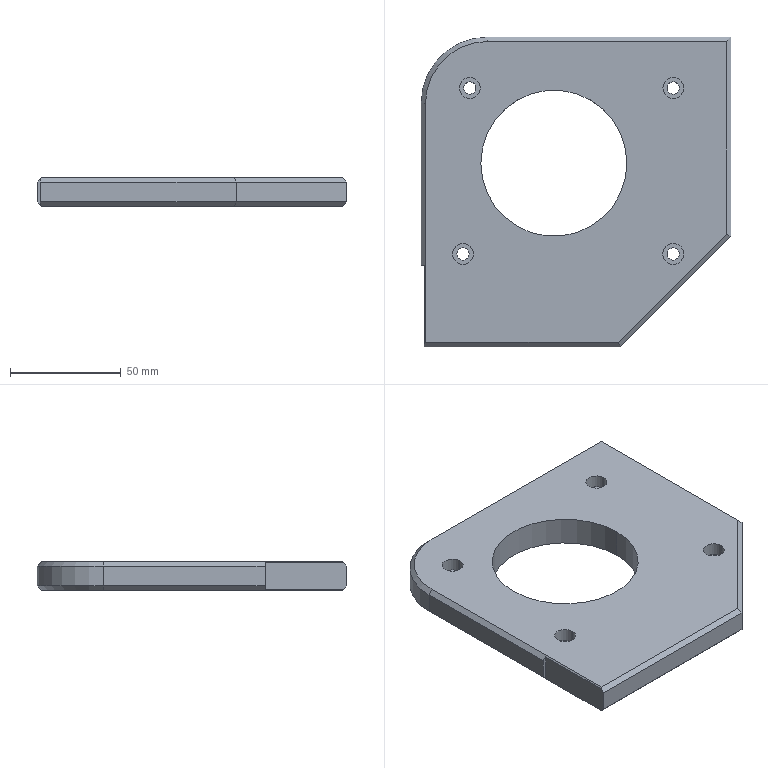Part | Creo | 1 solid | 44 faces | box 140 x 140 x 13 mm | volume 186564 mm3 | plane 23 | cylinder 19 | cone 2 | commonest cylinder face diameters 5.5 x8 9.5 x8 66 x2 60 x1
STEP:
#1=CARTESIAN_POINT('',(196.5,-375.005,-22.));
#2=VERTEX_POINT('',#1);
#3=CARTESIAN_POINT('',(196.5,-375.005,-13.));
#4=VERTEX_POINT('',#3);
#5=CARTESIAN_POINT('',(196.5,-375.005,-22.));
#6=DIRECTION('',(0.,0.,1.));
#7=VECTOR('',#6,9.);
#8=LINE('',#5,#7);
#9=EDGE_CURVE('',#2,#4,#8,.T.);
#10=ORIENTED_EDGE('',*,*,#9,.T.);
#11=CARTESIAN_POINT('',(285.,-375.005,-13.));
#12=VERTEX_POINT('',#11);
#13=CARTESIAN_POINT('',(196.5,-375.005,-13.));
#14=DIRECTION('',(1.,0.,0.));
#15=VECTOR('',#14,88.5);
#16=LINE('',#13,#15);
#17=EDGE_CURVE('',#4,#12,#16,.T.);
#18=ORIENTED_EDGE('',*,*,#17,.T.);
#19=CARTESIAN_POINT('',(285.,-375.005,-22.));
#20=VERTEX_POINT('',#19);
#21=CARTESIAN_POINT('',(285.,-375.005,-13.));
#22=DIRECTION('',(0.,0.,-1.));
#23=VECTOR('',#22,9.);
#24=LINE('',#21,#23);
#25=EDGE_CURVE('',#12,#20,#24,.T.);
#26=ORIENTED_EDGE('',*,*,#25,.T.);
#27=CARTESIAN_POINT('',(285.,-375.005,-22.));
#28=DIRECTION('',(-1.,0.,0.));
#29=VECTOR('',#28,88.5);
#30=LINE('',#27,#29);
#31=EDGE_CURVE('',#20,#2,#30,.T.);
#32=ORIENTED_EDGE('',*,*,#31,.T.);
#33=EDGE_LOOP('',(#10,#18,#26,#32));
#34=FACE_OUTER_BOUND('',#33,.F.);
#35=CARTESIAN_POINT('',(-265.,-375.005,-187.));
#36=DIRECTION('',(0.,-1.,0.));
#37=DIRECTION('',(0.,0.,1.));
#38=AXIS2_PLACEMENT_3D('',#35,#36,#37);
#39=PLANE('',#38);
#40=ADVANCED_FACE('',(#34),#39,.T.);
#41=CARTESIAN_POINT('',(196.5,-338.005,-11.5));
#42=VERTEX_POINT('',#41);
#43=CARTESIAN_POINT('',(196.5,-338.005,-23.5));
#44=VERTEX_POINT('',#43);
#45=CARTESIAN_POINT('',(196.5,-338.005,-11.5));
#46=DIRECTION('',(0.,0.,-1.));
#47=VECTOR('',#46,12.);
#48=LINE('',#45,#47);
#49=EDGE_CURVE('',#42,#44,#48,.T.);
#50=ORIENTED_EDGE('',*,*,#49,.F.);
#51=CARTESIAN_POINT('',(196.5,-373.505,-11.5));
#52=VERTEX_POINT('',#51);
#53=CARTESIAN_POINT('',(196.5,-338.005,-11.5));
#54=DIRECTION('',(0.,-1.,0.));
#55=VECTOR('',#54,35.5);
#56=LINE('',#53,#55);
#57=EDGE_CURVE('',#42,#52,#56,.T.);
#58=ORIENTED_EDGE('',*,*,#57,.T.);
#59=CARTESIAN_POINT('',(196.5,-375.005,-13.));
#60=DIRECTION('',(0.,0.7071,0.7071));
#61=VECTOR('',#60,2.121);
#62=LINE('',#59,#61);
#63=EDGE_CURVE('',#4,#52,#62,.T.);
#64=ORIENTED_EDGE('',*,*,#63,.F.);
#65=ORIENTED_EDGE('',*,*,#9,.F.);
#66=CARTESIAN_POINT('',(196.5,-373.505,-23.5));
#67=VERTEX_POINT('',#66);
#68=CARTESIAN_POINT('',(196.5,-373.505,-23.5));
#69=DIRECTION('',(0.,-0.7071,0.7071));
#70=VECTOR('',#69,2.121);
#71=LINE('',#68,#70);
#72=EDGE_CURVE('',#67,#2,#71,.T.);
#73=ORIENTED_EDGE('',*,*,#72,.F.);
#74=CARTESIAN_POINT('',(196.5,-373.505,-23.5));
#75=DIRECTION('',(0.,1.,0.));
#76=VECTOR('',#75,35.5);
#77=LINE('',#74,#76);
#78=EDGE_CURVE('',#67,#44,#77,.T.);
#79=ORIENTED_EDGE('',*,*,#78,.T.);
#80=EDGE_LOOP('',(#50,#58,#64,#65,#73,#79));
#81=FACE_OUTER_BOUND('',#80,.F.);
#82=CARTESIAN_POINT('',(196.5,-394.005,172.076));
#83=DIRECTION('',(1.,0.,0.));
#84=DIRECTION('',(0.,0.,-1.));
#85=AXIS2_PLACEMENT_3D('',#82,#83,#84);
#86=PLANE('',#85);
#87=ADVANCED_FACE('',(#81),#86,.F.);
#88=CARTESIAN_POINT('',(195.,-338.005,-13.));
#89=VERTEX_POINT('',#88);
#90=CARTESIAN_POINT('',(195.,-338.005,-22.));
#91=VERTEX_POINT('',#90);
#92=CARTESIAN_POINT('',(195.,-338.005,-13.));
#93=DIRECTION('',(0.,0.,-1.));
#94=VECTOR('',#93,9.);
#95=LINE('',#92,#94);
#96=EDGE_CURVE('',#89,#91,#95,.T.);
#97=ORIENTED_EDGE('',*,*,#96,.F.);
#98=CARTESIAN_POINT('',(196.5,-338.005,-11.5));
#99=DIRECTION('',(-0.7071,0.,-0.7071));
#100=VECTOR('',#99,2.121);
#101=LINE('',#98,#100);
#102=EDGE_CURVE('',#42,#89,#101,.T.);
#103=ORIENTED_EDGE('',*,*,#102,.F.);
#104=ORIENTED_EDGE('',*,*,#49,.T.);
#105=CARTESIAN_POINT('',(195.,-338.005,-22.));
#106=DIRECTION('',(0.7071,0.,-0.7071));
#107=VECTOR('',#106,2.121);
#108=LINE('',#105,#107);
#109=EDGE_CURVE('',#91,#44,#108,.T.);
#110=ORIENTED_EDGE('',*,*,#109,.F.);
#111=EDGE_LOOP('',(#97,#103,#104,#110));
#112=FACE_OUTER_BOUND('',#111,.F.);
#113=CARTESIAN_POINT('',(175.,-338.005,-2.));
#114=DIRECTION('',(0.,-1.,0.));
#115=DIRECTION('',(1.,0.,0.));
#116=AXIS2_PLACEMENT_3D('',#113,#114,#115);
#117=PLANE('',#116);
#118=ADVANCED_FACE('',(#112),#117,.T.);
#119=CARTESIAN_POINT('',(195.,-265.005,-22.));
#120=VERTEX_POINT('',#119);
#121=CARTESIAN_POINT('',(195.,-265.005,-13.));
#122=VERTEX_POINT('',#121);
#123=CARTESIAN_POINT('',(195.,-265.005,-22.));
#124=DIRECTION('',(0.,0.,1.));
#125=VECTOR('',#124,9.);
#126=LINE('',#123,#125);
#127=EDGE_CURVE('',#120,#122,#126,.T.);
#128=ORIENTED_EDGE('',*,*,#127,.T.);
#129=CARTESIAN_POINT('',(195.,-265.005,-13.));
#130=DIRECTION('',(0.,-1.,0.));
#131=VECTOR('',#130,73.);
#132=LINE('',#129,#131);
#133=EDGE_CURVE('',#122,#89,#132,.T.);
#134=ORIENTED_EDGE('',*,*,#133,.T.);
#135=ORIENTED_EDGE('',*,*,#96,.T.);
#136=CARTESIAN_POINT('',(195.,-338.005,-22.));
#137=DIRECTION('',(0.,1.,0.));
#138=VECTOR('',#137,73.);
#139=LINE('',#136,#138);
#140=EDGE_CURVE('',#91,#120,#139,.T.);
#141=ORIENTED_EDGE('',*,*,#140,.T.);
#142=EDGE_LOOP('',(#128,#134,#135,#141));
#143=FACE_OUTER_BOUND('',#142,.F.);
#144=CARTESIAN_POINT('',(195.,-0.004699,-23.));
#145=DIRECTION('',(1.,0.,0.));
#146=DIRECTION('',(0.,-1.,0.));
#147=AXIS2_PLACEMENT_3D('',#144,#145,#146);
#148=PLANE('',#147);
#149=ADVANCED_FACE('',(#143),#148,.F.);
#150=CARTESIAN_POINT('',(225.,-235.005,-13.));
#151=VERTEX_POINT('',#150);
#152=CARTESIAN_POINT('',(225.,-235.005,-22.));
#153=VERTEX_POINT('',#152);
#154=CARTESIAN_POINT('',(225.,-235.005,-13.));
#155=DIRECTION('',(0.,0.,-1.));
#156=VECTOR('',#155,9.);
#157=LINE('',#154,#156);
#158=EDGE_CURVE('',#151,#153,#157,.T.);
#159=ORIENTED_EDGE('',*,*,#158,.F.);
#160=CARTESIAN_POINT('',(225.,-265.005,-13.));
#161=DIRECTION('',(0.,0.,1.));
#162=DIRECTION('',(0.,1.,0.));
#163=AXIS2_PLACEMENT_3D('',#160,#161,#162);
#164=CIRCLE('',#163,30.);
#165=EDGE_CURVE('',#151,#122,#164,.T.);
#166=ORIENTED_EDGE('',*,*,#165,.T.);
#167=ORIENTED_EDGE('',*,*,#127,.F.);
#168=CARTESIAN_POINT('',(225.,-265.005,-22.));
#169=DIRECTION('',(0.,0.,-1.));
#170=DIRECTION('',(-1.,0.,0.));
#171=AXIS2_PLACEMENT_3D('',#168,#169,#170);
#172=CIRCLE('',#171,30.);
#173=EDGE_CURVE('',#120,#153,#172,.T.);
#174=ORIENTED_EDGE('',*,*,#173,.T.);
#175=EDGE_LOOP('',(#159,#166,#167,#174));
#176=FACE_OUTER_BOUND('',#175,.F.);
#177=CARTESIAN_POINT('',(225.,-265.005,-12.));
#178=DIRECTION('',(0.,0.,1.));
#179=DIRECTION('',(-1.,0.,0.));
#180=AXIS2_PLACEMENT_3D('',#177,#178,#179);
#181=CYLINDRICAL_SURFACE('',#180,30.);
#182=ADVANCED_FACE('',(#176),#181,.T.);
#183=CARTESIAN_POINT('',(335.,-235.005,-22.));
#184=VERTEX_POINT('',#183);
#185=CARTESIAN_POINT('',(335.,-235.005,-13.));
#186=VERTEX_POINT('',#185);
#187=CARTESIAN_POINT('',(335.,-235.005,-22.));
#188=DIRECTION('',(0.,0.,1.));
#189=VECTOR('',#188,9.);
#190=LINE('',#187,#189);
#191=EDGE_CURVE('',#184,#186,#190,.T.);
#192=ORIENTED_EDGE('',*,*,#191,.T.);
#193=CARTESIAN_POINT('',(335.,-235.005,-13.));
#194=DIRECTION('',(-1.,0.,0.));
#195=VECTOR('',#194,110.);
#196=LINE('',#193,#195);
#197=EDGE_CURVE('',#186,#151,#196,.T.);
#198=ORIENTED_EDGE('',*,*,#197,.T.);
#199=ORIENTED_EDGE('',*,*,#158,.T.);
#200=CARTESIAN_POINT('',(225.,-235.005,-22.));
#201=DIRECTION('',(1.,0.,0.));
#202=VECTOR('',#201,110.);
#203=LINE('',#200,#202);
#204=EDGE_CURVE('',#153,#184,#203,.T.);
#205=ORIENTED_EDGE('',*,*,#204,.T.);
#206=EDGE_LOOP('',(#192,#198,#199,#205));
#207=FACE_OUTER_BOUND('',#206,.F.);
#208=CARTESIAN_POINT('',(245.,-235.005,-12.));
#209=DIRECTION('',(0.,1.,0.));
#210=DIRECTION('',(0.,0.,-1.));
#211=AXIS2_PLACEMENT_3D('',#208,#209,#210);
#212=PLANE('',#211);
#213=ADVANCED_FACE('',(#207),#212,.T.);
#214=CARTESIAN_POINT('',(335.,-325.005,-22.));
#215=VERTEX_POINT('',#214);
#216=CARTESIAN_POINT('',(335.,-325.005,-13.));
#217=VERTEX_POINT('',#216);
#218=CARTESIAN_POINT('',(335.,-325.005,-22.));
#219=DIRECTION('',(0.,0.,1.));
#220=VECTOR('',#219,9.);
#221=LINE('',#218,#220);
#222=EDGE_CURVE('',#215,#217,#221,.T.);
#223=ORIENTED_EDGE('',*,*,#222,.T.);
#224=CARTESIAN_POINT('',(335.,-325.005,-13.));
#225=DIRECTION('',(0.,1.,0.));
#226=VECTOR('',#225,90.);
#227=LINE('',#224,#226);
#228=EDGE_CURVE('',#217,#186,#227,.T.);
#229=ORIENTED_EDGE('',*,*,#228,.T.);
#230=ORIENTED_EDGE('',*,*,#191,.F.);
#231=CARTESIAN_POINT('',(335.,-235.005,-22.));
#232=DIRECTION('',(0.,-1.,0.));
#233=VECTOR('',#232,90.);
#234=LINE('',#231,#233);
#235=EDGE_CURVE('',#184,#215,#234,.T.);
#236=ORIENTED_EDGE('',*,*,#235,.T.);
#237=EDGE_LOOP('',(#223,#229,#230,#236));
#238=FACE_OUTER_BOUND('',#237,.F.);
#239=CARTESIAN_POINT('',(335.,-50.005,-27.));
#240=DIRECTION('',(1.,0.,0.));
#241=DIRECTION('',(0.,-1.,0.));
#242=AXIS2_PLACEMENT_3D('',#239,#240,#241);
#243=PLANE('',#242);
#244=ADVANCED_FACE('',(#238),#243,.T.);
#245=ORIENTED_EDGE('',*,*,#25,.F.);
#246=CARTESIAN_POINT('',(285.,-375.005,-13.));
#247=DIRECTION('',(0.7071,0.7071,0.));
#248=VECTOR('',#247,70.711);
#249=LINE('',#246,#248);
#250=EDGE_CURVE('',#12,#217,#249,.T.);
#251=ORIENTED_EDGE('',*,*,#250,.T.);
#252=ORIENTED_EDGE('',*,*,#222,.F.);
#253=CARTESIAN_POINT('',(335.,-325.005,-22.));
#254=DIRECTION('',(-0.7071,-0.7071,0.));
#255=VECTOR('',#254,70.711);
#256=LINE('',#253,#255);
#257=EDGE_CURVE('',#215,#20,#256,.T.);
#258=ORIENTED_EDGE('',*,*,#257,.T.);
#259=EDGE_LOOP('',(#245,#251,#252,#258));
#260=FACE_OUTER_BOUND('',#259,.F.);
#261=CARTESIAN_POINT('',(335.,-325.005,-27.));
#262=DIRECTION('',(-0.7071,0.7071,0.));
#263=DIRECTION('',(0.,0.,-1.));
#264=AXIS2_PLACEMENT_3D('',#261,#262,#263);
#265=PLANE('',#264);
#266=ADVANCED_FACE('',(#260),#265,.F.);
#267=CARTESIAN_POINT('',(333.,-324.176,-11.));
#268=VERTEX_POINT('',#267);
#269=CARTESIAN_POINT('',(333.,-324.176,-11.));
#270=DIRECTION('',(0.6786,-0.2811,-0.6786));
#271=VECTOR('',#270,2.947);
#272=LINE('',#269,#271);
#273=EDGE_CURVE('',#268,#217,#272,.T.);
#274=ORIENTED_EDGE('',*,*,#273,.T.);
#275=ORIENTED_EDGE('',*,*,#250,.F.);
#276=CARTESIAN_POINT('',(284.172,-373.005,-11.));
#277=VERTEX_POINT('',#276);
#278=CARTESIAN_POINT('',(284.172,-373.005,-11.));
#279=DIRECTION('',(0.2811,-0.6786,-0.6786));
#280=VECTOR('',#279,2.947);
#281=LINE('',#278,#280);
#282=EDGE_CURVE('',#277,#12,#281,.T.);
#283=ORIENTED_EDGE('',*,*,#282,.F.);
#284=CARTESIAN_POINT('',(284.172,-373.005,-11.));
#285=DIRECTION('',(0.7071,0.7071,0.));
#286=VECTOR('',#285,69.054);
#287=LINE('',#284,#286);
#288=EDGE_CURVE('',#277,#268,#287,.T.);
#289=ORIENTED_EDGE('',*,*,#288,.T.);
#290=EDGE_LOOP('',(#274,#275,#283,#289));
#291=FACE_OUTER_BOUND('',#290,.F.);
#292=CARTESIAN_POINT('',(299.836,-357.34,-11.));
#293=DIRECTION('',(0.5,-0.5,0.7071));
#294=DIRECTION('',(-0.7071,-0.7071,0.));
#295=AXIS2_PLACEMENT_3D('',#292,#293,#294);
#296=PLANE('',#295);
#297=ADVANCED_FACE('',(#291),#296,.T.);
#298=ORIENTED_EDGE('',*,*,#228,.F.);
#299=ORIENTED_EDGE('',*,*,#273,.F.);
#300=CARTESIAN_POINT('',(333.,-237.005,-11.));
#301=VERTEX_POINT('',#300);
#302=CARTESIAN_POINT('',(333.,-237.005,-11.));
#303=DIRECTION('',(0.,-1.,0.));
#304=VECTOR('',#303,87.172);
#305=LINE('',#302,#304);
#306=EDGE_CURVE('',#301,#268,#305,.T.);
#307=ORIENTED_EDGE('',*,*,#306,.F.);
#308=CARTESIAN_POINT('',(333.,-237.005,-11.));
#309=DIRECTION('',(0.5774,0.5774,-0.5774));
#310=VECTOR('',#309,3.464);
#311=LINE('',#308,#310);
#312=EDGE_CURVE('',#301,#186,#311,.T.);
#313=ORIENTED_EDGE('',*,*,#312,.T.);
#314=EDGE_LOOP('',(#298,#299,#307,#313));
#315=FACE_OUTER_BOUND('',#314,.F.);
#316=CARTESIAN_POINT('',(333.,-302.505,-11.));
#317=DIRECTION('',(-0.7071,0.,-0.7071));
#318=DIRECTION('',(0.,1.,0.));
#319=AXIS2_PLACEMENT_3D('',#316,#317,#318);
#320=PLANE('',#319);
#321=ADVANCED_FACE('',(#315),#320,.F.);
#322=ORIENTED_EDGE('',*,*,#306,.T.);
#323=ORIENTED_EDGE('',*,*,#288,.F.);
#324=CARTESIAN_POINT('',(197.,-373.005,-11.));
#325=VERTEX_POINT('',#324);
#326=CARTESIAN_POINT('',(284.172,-373.005,-11.));
#327=DIRECTION('',(-1.,0.,0.));
#328=VECTOR('',#327,87.172);
#329=LINE('',#326,#328);
#330=EDGE_CURVE('',#277,#325,#329,.T.);
#331=ORIENTED_EDGE('',*,*,#330,.T.);
#332=CARTESIAN_POINT('',(197.,-265.005,-11.));
#333=VERTEX_POINT('',#332);
#334=CARTESIAN_POINT('',(197.,-373.005,-11.));
#335=DIRECTION('',(0.,1.,0.));
#336=VECTOR('',#335,108.);
#337=LINE('',#334,#336);
#338=EDGE_CURVE('',#325,#333,#337,.T.);
#339=ORIENTED_EDGE('',*,*,#338,.T.);
#340=CARTESIAN_POINT('',(225.,-237.005,-11.));
#341=VERTEX_POINT('',#340);
#342=CARTESIAN_POINT('',(225.,-265.005,-11.));
#343=DIRECTION('',(0.,0.,1.));
#344=DIRECTION('',(0.,1.,0.));
#345=AXIS2_PLACEMENT_3D('',#342,#343,#344);
#346=CIRCLE('',#345,28.);
#347=EDGE_CURVE('',#341,#333,#346,.T.);
#348=ORIENTED_EDGE('',*,*,#347,.F.);
#349=CARTESIAN_POINT('',(225.,-237.005,-11.));
#350=DIRECTION('',(1.,0.,0.));
#351=VECTOR('',#350,108.);
#352=LINE('',#349,#351);
#353=EDGE_CURVE('',#341,#301,#352,.T.);
#354=ORIENTED_EDGE('',*,*,#353,.T.);
#355=EDGE_LOOP('',(#322,#323,#331,#339,#348,#354));
#356=FACE_OUTER_BOUND('',#355,.F.);
#357=CARTESIAN_POINT('',(313.699,-333.009,-11.));
#358=VERTEX_POINT('',#357);
#359=CARTESIAN_POINT('',(304.199,-333.009,-11.));
#360=VERTEX_POINT('',#359);
#361=CARTESIAN_POINT('',(308.949,-333.009,-11.));
#362=DIRECTION('',(0.,0.,-1.));
#363=DIRECTION('',(1.,0.,0.));
#364=AXIS2_PLACEMENT_3D('',#361,#362,#363);
#365=CIRCLE('',#364,4.75);
#366=EDGE_CURVE('',#358,#360,#365,.T.);
#367=ORIENTED_EDGE('',*,*,#366,.F.);
#368=CARTESIAN_POINT('',(308.949,-333.009,-11.));
#369=DIRECTION('',(0.,0.,-1.));
#370=DIRECTION('',(-1.,0.,0.));
#371=AXIS2_PLACEMENT_3D('',#368,#369,#370);
#372=CIRCLE('',#371,4.75);
#373=EDGE_CURVE('',#360,#358,#372,.T.);
#374=ORIENTED_EDGE('',*,*,#373,.F.);
#375=EDGE_LOOP('',(#367,#374));
#376=FACE_BOUND('',#375,.F.);
#377=CARTESIAN_POINT('',(221.75,-258.009,-11.));
#378=VERTEX_POINT('',#377);
#379=CARTESIAN_POINT('',(212.25,-258.009,-11.));
#380=VERTEX_POINT('',#379);
#381=CARTESIAN_POINT('',(217.,-258.009,-11.));
#382=DIRECTION('',(0.,0.,-1.));
#383=DIRECTION('',(1.,0.,0.));
#384=AXIS2_PLACEMENT_3D('',#381,#382,#383);
#385=CIRCLE('',#384,4.75);
#386=EDGE_CURVE('',#378,#380,#385,.T.);
#387=ORIENTED_EDGE('',*,*,#386,.F.);
#388=CARTESIAN_POINT('',(217.,-258.009,-11.));
#389=DIRECTION('',(0.,0.,-1.));
#390=DIRECTION('',(-1.,0.,0.));
#391=AXIS2_PLACEMENT_3D('',#388,#389,#390);
#392=CIRCLE('',#391,4.75);
#393=EDGE_CURVE('',#380,#378,#392,.T.);
#394=ORIENTED_EDGE('',*,*,#393,.F.);
#395=EDGE_LOOP('',(#387,#394));
#396=FACE_BOUND('',#395,.F.);
#397=CARTESIAN_POINT('',(313.75,-258.009,-11.));
#398=VERTEX_POINT('',#397);
#399=CARTESIAN_POINT('',(304.25,-258.009,-11.));
#400=VERTEX_POINT('',#399);
#401=CARTESIAN_POINT('',(309.,-258.009,-11.));
#402=DIRECTION('',(0.,0.,-1.));
#403=DIRECTION('',(1.,0.,0.));
#404=AXIS2_PLACEMENT_3D('',#401,#402,#403);
#405=CIRCLE('',#404,4.75);
#406=EDGE_CURVE('',#398,#400,#405,.T.);
#407=ORIENTED_EDGE('',*,*,#406,.F.);
#408=CARTESIAN_POINT('',(309.,-258.009,-11.));
#409=DIRECTION('',(0.,0.,-1.));
#410=DIRECTION('',(-1.,0.,0.));
#411=AXIS2_PLACEMENT_3D('',#408,#409,#410);
#412=CIRCLE('',#411,4.75);
#413=EDGE_CURVE('',#400,#398,#412,.T.);
#414=ORIENTED_EDGE('',*,*,#413,.F.);
#415=EDGE_LOOP('',(#407,#414));
#416=FACE_BOUND('',#415,.F.);
#417=CARTESIAN_POINT('',(218.699,-333.009,-11.));
#418=VERTEX_POINT('',#417);
#419=CARTESIAN_POINT('',(209.199,-333.009,-11.));
#420=VERTEX_POINT('',#419);
#421=CARTESIAN_POINT('',(213.949,-333.009,-11.));
#422=DIRECTION('',(0.,0.,-1.));
#423=DIRECTION('',(1.,0.,0.));
#424=AXIS2_PLACEMENT_3D('',#421,#422,#423);
#425=CIRCLE('',#424,4.75);
#426=EDGE_CURVE('',#418,#420,#425,.T.);
#427=ORIENTED_EDGE('',*,*,#426,.F.);
#428=CARTESIAN_POINT('',(213.949,-333.009,-11.));
#429=DIRECTION('',(0.,0.,-1.));
#430=DIRECTION('',(-1.,0.,0.));
#431=AXIS2_PLACEMENT_3D('',#428,#429,#430);
#432=CIRCLE('',#431,4.75);
#433=EDGE_CURVE('',#420,#418,#432,.T.);
#434=ORIENTED_EDGE('',*,*,#433,.F.);
#435=EDGE_LOOP('',(#427,#434));
#436=FACE_BOUND('',#435,.F.);
#437=CARTESIAN_POINT('',(288.,-292.005,-11.));
#438=VERTEX_POINT('',#437);
#439=CARTESIAN_POINT('',(222.,-292.005,-11.));
#440=VERTEX_POINT('',#439);
#441=CARTESIAN_POINT('',(255.,-292.005,-11.));
#442=DIRECTION('',(0.,0.,-1.));
#443=DIRECTION('',(1.,0.,0.));
#444=AXIS2_PLACEMENT_3D('',#441,#442,#443);
#445=CIRCLE('',#444,33.);
#446=EDGE_CURVE('',#438,#440,#445,.T.);
#447=ORIENTED_EDGE('',*,*,#446,.F.);
#448=CARTESIAN_POINT('',(255.,-292.005,-11.));
#449=DIRECTION('',(0.,0.,-1.));
#450=DIRECTION('',(-1.,0.,0.));
#451=AXIS2_PLACEMENT_3D('',#448,#449,#450);
#452=CIRCLE('',#451,33.);
#453=EDGE_CURVE('',#440,#438,#452,.T.);
#454=ORIENTED_EDGE('',*,*,#453,.F.);
#455=EDGE_LOOP('',(#447,#454));
#456=FACE_BOUND('',#455,.F.);
#457=CARTESIAN_POINT('',(245.,-302.505,-11.));
#458=DIRECTION('',(0.,0.,1.));
#459=DIRECTION('',(-1.,0.,0.));
#460=AXIS2_PLACEMENT_3D('',#457,#458,#459);
#461=PLANE('',#460);
#462=ADVANCED_FACE('',(#356,#376,#396,#416,#436,#456),#461,.T.);
#463=ORIENTED_EDGE('',*,*,#330,.F.);
#464=ORIENTED_EDGE('',*,*,#282,.T.);
#465=ORIENTED_EDGE('',*,*,#17,.F.);
#466=ORIENTED_EDGE('',*,*,#63,.T.);
#467=CARTESIAN_POINT('',(196.5,-373.505,-11.5));
#468=DIRECTION('',(0.5774,0.5774,0.5774));
#469=VECTOR('',#468,0.866);
#470=LINE('',#467,#469);
#471=EDGE_CURVE('',#52,#325,#470,.T.);
#472=ORIENTED_EDGE('',*,*,#471,.T.);
#473=EDGE_LOOP('',(#463,#464,#465,#466,#472));
#474=FACE_OUTER_BOUND('',#473,.F.);
#475=CARTESIAN_POINT('',(245.,-373.005,-11.));
#476=DIRECTION('',(0.,0.7071,-0.7071));
#477=DIRECTION('',(1.,0.,0.));
#478=AXIS2_PLACEMENT_3D('',#475,#476,#477);
#479=PLANE('',#478);
#480=ADVANCED_FACE('',(#474),#479,.F.);
#481=ORIENTED_EDGE('',*,*,#471,.F.);
#482=ORIENTED_EDGE('',*,*,#57,.F.);
#483=ORIENTED_EDGE('',*,*,#102,.T.);
#484=ORIENTED_EDGE('',*,*,#133,.F.);
#485=CARTESIAN_POINT('',(195.,-265.005,-13.));
#486=DIRECTION('',(0.7071,0.,0.7071));
#487=VECTOR('',#486,2.828);
#488=LINE('',#485,#487);
#489=EDGE_CURVE('',#122,#333,#488,.T.);
#490=ORIENTED_EDGE('',*,*,#489,.T.);
#491=ORIENTED_EDGE('',*,*,#338,.F.);
#492=EDGE_LOOP('',(#481,#482,#483,#484,#490,#491));
#493=FACE_OUTER_BOUND('',#492,.F.);
#494=CARTESIAN_POINT('',(197.,-302.505,-11.));
#495=DIRECTION('',(-0.7071,0.,0.7071));
#496=DIRECTION('',(0.,1.,0.));
#497=AXIS2_PLACEMENT_3D('',#494,#495,#496);
#498=PLANE('',#497);
#499=ADVANCED_FACE('',(#493),#498,.T.);
#500=ORIENTED_EDGE('',*,*,#489,.F.);
#501=ORIENTED_EDGE('',*,*,#165,.F.);
#502=CARTESIAN_POINT('',(225.,-237.005,-11.));
#503=DIRECTION('',(0.,0.7071,-0.7071));
#504=VECTOR('',#503,2.828);
#505=LINE('',#502,#504);
#506=EDGE_CURVE('',#341,#151,#505,.T.);
#507=ORIENTED_EDGE('',*,*,#506,.F.);
#508=ORIENTED_EDGE('',*,*,#347,.T.);
#509=EDGE_LOOP('',(#500,#501,#507,#508));
#510=FACE_OUTER_BOUND('',#509,.F.);
#511=CARTESIAN_POINT('',(225.,-265.005,-12.));
#512=DIRECTION('',(0.,0.,-1.));
#513=DIRECTION('',(-1.,0.,0.));
#514=AXIS2_PLACEMENT_3D('',#511,#512,#513);
#515=CONICAL_SURFACE('',#514,29.,45.);
#516=ADVANCED_FACE('',(#510),#515,.T.);
#517=ORIENTED_EDGE('',*,*,#312,.F.);
#518=ORIENTED_EDGE('',*,*,#353,.F.);
#519=ORIENTED_EDGE('',*,*,#506,.T.);
#520=ORIENTED_EDGE('',*,*,#197,.F.);
#521=EDGE_LOOP('',(#517,#518,#519,#520));
#522=FACE_OUTER_BOUND('',#521,.F.);
#523=CARTESIAN_POINT('',(245.,-237.005,-11.));
#524=DIRECTION('',(0.,-0.7071,-0.7071));
#525=DIRECTION('',(-1.,0.,0.));
#526=AXIS2_PLACEMENT_3D('',#523,#524,#525);
#527=PLANE('',#526);
#528=ADVANCED_FACE('',(#522),#527,.F.);
#529=CARTESIAN_POINT('',(304.199,-333.009,-17.));
#530=VERTEX_POINT('',#529);
#531=CARTESIAN_POINT('',(313.699,-333.009,-17.));
#532=VERTEX_POINT('',#531);
#533=CARTESIAN_POINT('',(308.949,-333.009,-17.));
#534=DIRECTION('',(0.,0.,1.));
#535=DIRECTION('',(-1.,0.,0.));
#536=AXIS2_PLACEMENT_3D('',#533,#534,#535);
#537=CIRCLE('',#536,4.75);
#538=EDGE_CURVE('',#530,#532,#537,.T.);
#539=ORIENTED_EDGE('',*,*,#538,.T.);
#540=CARTESIAN_POINT('',(313.699,-333.009,-17.));
#541=DIRECTION('',(0.,0.,1.));
#542=VECTOR('',#541,6.);
#543=LINE('',#540,#542);
#544=EDGE_CURVE('',#532,#358,#543,.T.);
#545=ORIENTED_EDGE('',*,*,#544,.T.);
#546=ORIENTED_EDGE('',*,*,#366,.T.);
#547=CARTESIAN_POINT('',(304.199,-333.009,-17.));
#548=DIRECTION('',(0.,0.,1.));
#549=VECTOR('',#548,6.);
#550=LINE('',#547,#549);
#551=EDGE_CURVE('',#530,#360,#550,.T.);
#552=ORIENTED_EDGE('',*,*,#551,.F.);
#553=EDGE_LOOP('',(#539,#545,#546,#552));
#554=FACE_OUTER_BOUND('',#553,.F.);
#555=CARTESIAN_POINT('',(308.949,-333.009,-11.));
#556=DIRECTION('',(0.,0.,1.));
#557=DIRECTION('',(1.,0.,0.));
#558=AXIS2_PLACEMENT_3D('',#555,#556,#557);
#559=CYLINDRICAL_SURFACE('',#558,4.75);
#560=ADVANCED_FACE('',(#554),#559,.F.);
#561=CARTESIAN_POINT('',(308.949,-333.009,-17.));
#562=DIRECTION('',(0.,0.,1.));
#563=DIRECTION('',(1.,0.,0.));
#564=AXIS2_PLACEMENT_3D('',#561,#562,#563);
#565=CIRCLE('',#564,4.75);
#566=EDGE_CURVE('',#532,#530,#565,.T.);
#567=ORIENTED_EDGE('',*,*,#566,.F.);
#568=ORIENTED_EDGE('',*,*,#538,.F.);
#569=EDGE_LOOP('',(#567,#568));
#570=FACE_OUTER_BOUND('',#569,.F.);
#571=CARTESIAN_POINT('',(311.699,-333.009,-17.));
#572=VERTEX_POINT('',#571);
#573=CARTESIAN_POINT('',(306.199,-333.009,-17.));
#574=VERTEX_POINT('',#573);
#575=CARTESIAN_POINT('',(308.949,-333.009,-17.));
#576=DIRECTION('',(0.,0.,-1.));
#577=DIRECTION('',(1.,0.,0.));
#578=AXIS2_PLACEMENT_3D('',#575,#576,#577);
#579=CIRCLE('',#578,2.75);
#580=EDGE_CURVE('',#572,#574,#579,.T.);
#581=ORIENTED_EDGE('',*,*,#580,.F.);
#582=CARTESIAN_POINT('',(308.949,-333.009,-17.));
#583=DIRECTION('',(0.,0.,-1.));
#584=DIRECTION('',(-1.,0.,0.));
#585=AXIS2_PLACEMENT_3D('',#582,#583,#584);
#586=CIRCLE('',#585,2.75);
#587=EDGE_CURVE('',#574,#572,#586,.T.);
#588=ORIENTED_EDGE('',*,*,#587,.F.);
#589=EDGE_LOOP('',(#581,#588));
#590=FACE_BOUND('',#589,.F.);
#591=CARTESIAN_POINT('',(308.949,-328.259,-17.));
#592=DIRECTION('',(0.,0.,-1.));
#593=DIRECTION('',(-1.,0.,0.));
#594=AXIS2_PLACEMENT_3D('',#591,#592,#593);
#595=PLANE('',#594);
#596=ADVANCED_FACE('',(#570,#590),#595,.F.);
#597=CARTESIAN_POINT('',(306.199,-333.009,-24.));
#598=VERTEX_POINT('',#597);
#599=CARTESIAN_POINT('',(311.699,-333.009,-24.));
#600=VERTEX_POINT('',#599);
#601=CARTESIAN_POINT('',(308.949,-333.009,-24.));
#602=DIRECTION('',(0.,0.,1.));
#603=DIRECTION('',(-1.,0.,0.));
#604=AXIS2_PLACEMENT_3D('',#601,#602,#603);
#605=CIRCLE('',#604,2.75);
#606=EDGE_CURVE('',#598,#600,#605,.T.);
#607=ORIENTED_EDGE('',*,*,#606,.T.);
#608=CARTESIAN_POINT('',(311.699,-333.009,-24.));
#609=DIRECTION('',(0.,0.,1.));
#610=VECTOR('',#609,7.);
#611=LINE('',#608,#610);
#612=EDGE_CURVE('',#600,#572,#611,.T.);
#613=ORIENTED_EDGE('',*,*,#612,.T.);
#614=ORIENTED_EDGE('',*,*,#580,.T.);
#615=CARTESIAN_POINT('',(306.199,-333.009,-24.));
#616=DIRECTION('',(0.,0.,1.));
#617=VECTOR('',#616,7.);
#618=LINE('',#615,#617);
#619=EDGE_CURVE('',#598,#574,#618,.T.);
#620=ORIENTED_EDGE('',*,*,#619,.F.);
#621=EDGE_LOOP('',(#607,#613,#614,#620));
#622=FACE_OUTER_BOUND('',#621,.F.);
#623=CARTESIAN_POINT('',(308.949,-333.009,-11.));
#624=DIRECTION('',(0.,0.,1.));
#625=DIRECTION('',(1.,0.,0.));
#626=AXIS2_PLACEMENT_3D('',#623,#624,#625);
#627=CYLINDRICAL_SURFACE('',#626,2.75);
#628=ADVANCED_FACE('',(#622),#627,.F.);
#629=CARTESIAN_POINT('',(197.,-265.005,-24.));
#630=VERTEX_POINT('',#629);
#631=CARTESIAN_POINT('',(225.,-237.005,-24.));
#632=VERTEX_POINT('',#631);
#633=CARTESIAN_POINT('',(225.,-265.005,-24.));
#634=DIRECTION('',(0.,0.,-1.));
#635=DIRECTION('',(-1.,0.,0.));
#636=AXIS2_PLACEMENT_3D('',#633,#634,#635);
#637=CIRCLE('',#636,28.);
#638=EDGE_CURVE('',#630,#632,#637,.T.);
#639=ORIENTED_EDGE('',*,*,#638,.F.);
#640=CARTESIAN_POINT('',(197.,-373.005,-24.));
#641=VERTEX_POINT('',#640);
#642=CARTESIAN_POINT('',(197.,-265.005,-24.));
#643=DIRECTION('',(0.,-1.,0.));
#644=VECTOR('',#643,108.);
#645=LINE('',#642,#644);
#646=EDGE_CURVE('',#630,#641,#645,.T.);
#647=ORIENTED_EDGE('',*,*,#646,.T.);
#648=CARTESIAN_POINT('',(284.172,-373.005,-24.));
#649=VERTEX_POINT('',#648);
#650=CARTESIAN_POINT('',(197.,-373.005,-24.));
#651=DIRECTION('',(1.,0.,0.));
#652=VECTOR('',#651,87.172);
#653=LINE('',#650,#652);
#654=EDGE_CURVE('',#641,#649,#653,.T.);
#655=ORIENTED_EDGE('',*,*,#654,.T.);
#656=CARTESIAN_POINT('',(333.,-324.176,-24.));
#657=VERTEX_POINT('',#656);
#658=CARTESIAN_POINT('',(333.,-324.176,-24.));
#659=DIRECTION('',(-0.7071,-0.7071,0.));
#660=VECTOR('',#659,69.054);
#661=LINE('',#658,#660);
#662=EDGE_CURVE('',#657,#649,#661,.T.);
#663=ORIENTED_EDGE('',*,*,#662,.F.);
#664=CARTESIAN_POINT('',(333.,-237.005,-24.));
#665=VERTEX_POINT('',#664);
#666=CARTESIAN_POINT('',(333.,-324.176,-24.));
#667=DIRECTION('',(0.,1.,0.));
#668=VECTOR('',#667,87.172);
#669=LINE('',#666,#668);
#670=EDGE_CURVE('',#657,#665,#669,.T.);
#671=ORIENTED_EDGE('',*,*,#670,.T.);
#672=CARTESIAN_POINT('',(333.,-237.005,-24.));
#673=DIRECTION('',(-1.,0.,0.));
#674=VECTOR('',#673,108.);
#675=LINE('',#672,#674);
#676=EDGE_CURVE('',#665,#632,#675,.T.);
#677=ORIENTED_EDGE('',*,*,#676,.T.);
#678=EDGE_LOOP('',(#639,#647,#655,#663,#671,#677));
#679=FACE_OUTER_BOUND('',#678,.F.);
#680=ORIENTED_EDGE('',*,*,#606,.F.);
#681=CARTESIAN_POINT('',(308.949,-333.009,-24.));
#682=DIRECTION('',(0.,0.,1.));
#683=DIRECTION('',(1.,0.,0.));
#684=AXIS2_PLACEMENT_3D('',#681,#682,#683);
#685=CIRCLE('',#684,2.75);
#686=EDGE_CURVE('',#600,#598,#685,.T.);
#687=ORIENTED_EDGE('',*,*,#686,.F.);
#688=EDGE_LOOP('',(#680,#687));
#689=FACE_BOUND('',#688,.F.);
#690=CARTESIAN_POINT('',(214.25,-258.009,-24.));
#691=VERTEX_POINT('',#690);
#692=CARTESIAN_POINT('',(219.75,-258.009,-24.));
#693=VERTEX_POINT('',#692);
#694=CARTESIAN_POINT('',(217.,-258.009,-24.));
#695=DIRECTION('',(0.,0.,1.));
#696=DIRECTION('',(-1.,0.,0.));
#697=AXIS2_PLACEMENT_3D('',#694,#695,#696);
#698=CIRCLE('',#697,2.75);
#699=EDGE_CURVE('',#691,#693,#698,.T.);
#700=ORIENTED_EDGE('',*,*,#699,.F.);
#701=CARTESIAN_POINT('',(217.,-258.009,-24.));
#702=DIRECTION('',(0.,0.,1.));
#703=DIRECTION('',(1.,0.,0.));
#704=AXIS2_PLACEMENT_3D('',#701,#702,#703);
#705=CIRCLE('',#704,2.75);
#706=EDGE_CURVE('',#693,#691,#705,.T.);
#707=ORIENTED_EDGE('',*,*,#706,.F.);
#708=EDGE_LOOP('',(#700,#707));
#709=FACE_BOUND('',#708,.F.);
#710=CARTESIAN_POINT('',(306.25,-258.009,-24.));
#711=VERTEX_POINT('',#710);
#712=CARTESIAN_POINT('',(311.75,-258.009,-24.));
#713=VERTEX_POINT('',#712);
#714=CARTESIAN_POINT('',(309.,-258.009,-24.));
#715=DIRECTION('',(0.,0.,1.));
#716=DIRECTION('',(-1.,0.,0.));
#717=AXIS2_PLACEMENT_3D('',#714,#715,#716);
#718=CIRCLE('',#717,2.75);
#719=EDGE_CURVE('',#711,#713,#718,.T.);
#720=ORIENTED_EDGE('',*,*,#719,.F.);
#721=CARTESIAN_POINT('',(309.,-258.009,-24.));
#722=DIRECTION('',(0.,0.,1.));
#723=DIRECTION('',(1.,0.,0.));
#724=AXIS2_PLACEMENT_3D('',#721,#722,#723);
#725=CIRCLE('',#724,2.75);
#726=EDGE_CURVE('',#713,#711,#725,.T.);
#727=ORIENTED_EDGE('',*,*,#726,.F.);
#728=EDGE_LOOP('',(#720,#727));
#729=FACE_BOUND('',#728,.F.);
#730=CARTESIAN_POINT('',(211.199,-333.009,-24.));
#731=VERTEX_POINT('',#730);
#732=CARTESIAN_POINT('',(216.699,-333.009,-24.));
#733=VERTEX_POINT('',#732);
#734=CARTESIAN_POINT('',(213.949,-333.009,-24.));
#735=DIRECTION('',(0.,0.,1.));
#736=DIRECTION('',(-1.,0.,0.));
#737=AXIS2_PLACEMENT_3D('',#734,#735,#736);
#738=CIRCLE('',#737,2.75);
#739=EDGE_CURVE('',#731,#733,#738,.T.);
#740=ORIENTED_EDGE('',*,*,#739,.F.);
#741=CARTESIAN_POINT('',(213.949,-333.009,-24.));
#742=DIRECTION('',(0.,0.,1.));
#743=DIRECTION('',(1.,0.,0.));
#744=AXIS2_PLACEMENT_3D('',#741,#742,#743);
#745=CIRCLE('',#744,2.75);
#746=EDGE_CURVE('',#733,#731,#745,.T.);
#747=ORIENTED_EDGE('',*,*,#746,.F.);
#748=EDGE_LOOP('',(#740,#747));
#749=FACE_BOUND('',#748,.F.);
#750=CARTESIAN_POINT('',(222.,-292.005,-24.));
#751=VERTEX_POINT('',#750);
#752=CARTESIAN_POINT('',(288.,-292.005,-24.));
#753=VERTEX_POINT('',#752);
#754=CARTESIAN_POINT('',(255.,-292.005,-24.));
#755=DIRECTION('',(0.,0.,1.));
#756=DIRECTION('',(-1.,0.,0.));
#757=AXIS2_PLACEMENT_3D('',#754,#755,#756);
#758=CIRCLE('',#757,33.);
#759=EDGE_CURVE('',#751,#753,#758,.T.);
#760=ORIENTED_EDGE('',*,*,#759,.F.);
#761=CARTESIAN_POINT('',(255.,-292.005,-24.));
#762=DIRECTION('',(0.,0.,1.));
#763=DIRECTION('',(1.,0.,0.));
#764=AXIS2_PLACEMENT_3D('',#761,#762,#763);
#765=CIRCLE('',#764,33.);
#766=EDGE_CURVE('',#753,#751,#765,.T.);
#767=ORIENTED_EDGE('',*,*,#766,.F.);
#768=EDGE_LOOP('',(#760,#767));
#769=FACE_BOUND('',#768,.F.);
#770=CARTESIAN_POINT('',(245.,-302.505,-24.));
#771=DIRECTION('',(0.,0.,-1.));
#772=DIRECTION('',(1.,0.,0.));
#773=AXIS2_PLACEMENT_3D('',#770,#771,#772);
#774=PLANE('',#773);
#775=ADVANCED_FACE('',(#679,#689,#709,#729,#749,#769),#774,.T.);
#776=CARTESIAN_POINT('',(197.,-265.005,-24.));
#777=DIRECTION('',(-0.7071,0.,0.7071));
#778=VECTOR('',#777,2.828);
#779=LINE('',#776,#778);
#780=EDGE_CURVE('',#630,#120,#779,.T.);
#781=ORIENTED_EDGE('',*,*,#780,.F.);
#782=ORIENTED_EDGE('',*,*,#638,.T.);
#783=CARTESIAN_POINT('',(225.,-235.005,-22.));
#784=DIRECTION('',(0.,-0.7071,-0.7071));
#785=VECTOR('',#784,2.828);
#786=LINE('',#783,#785);
#787=EDGE_CURVE('',#153,#632,#786,.T.);
#788=ORIENTED_EDGE('',*,*,#787,.F.);
#789=ORIENTED_EDGE('',*,*,#173,.F.);
#790=EDGE_LOOP('',(#781,#782,#788,#789));
#791=FACE_OUTER_BOUND('',#790,.F.);
#792=CARTESIAN_POINT('',(225.,-265.005,-23.));
#793=DIRECTION('',(0.,0.,1.));
#794=DIRECTION('',(1.,0.,0.));
#795=AXIS2_PLACEMENT_3D('',#792,#793,#794);
#796=CONICAL_SURFACE('',#795,29.,45.);
#797=ADVANCED_FACE('',(#791),#796,.T.);
#798=ORIENTED_EDGE('',*,*,#109,.T.);
#799=ORIENTED_EDGE('',*,*,#78,.F.);
#800=CARTESIAN_POINT('',(196.5,-373.505,-23.5));
#801=DIRECTION('',(0.5774,0.5774,-0.5774));
#802=VECTOR('',#801,0.866);
#803=LINE('',#800,#802);
#804=EDGE_CURVE('',#67,#641,#803,.T.);
#805=ORIENTED_EDGE('',*,*,#804,.T.);
#806=ORIENTED_EDGE('',*,*,#646,.F.);
#807=ORIENTED_EDGE('',*,*,#780,.T.);
#808=ORIENTED_EDGE('',*,*,#140,.F.);
#809=EDGE_LOOP('',(#798,#799,#805,#806,#807,#808));
#810=FACE_OUTER_BOUND('',#809,.F.);
#811=CARTESIAN_POINT('',(197.,-302.505,-24.));
#812=DIRECTION('',(-0.7071,0.,-0.7071));
#813=DIRECTION('',(0.,-1.,0.));
#814=AXIS2_PLACEMENT_3D('',#811,#812,#813);
#815=PLANE('',#814);
#816=ADVANCED_FACE('',(#810),#815,.T.);
#817=ORIENTED_EDGE('',*,*,#31,.F.);
#818=CARTESIAN_POINT('',(284.172,-373.005,-24.));
#819=DIRECTION('',(0.2811,-0.6786,0.6786));
#820=VECTOR('',#819,2.947);
#821=LINE('',#818,#820);
#822=EDGE_CURVE('',#649,#20,#821,.T.);
#823=ORIENTED_EDGE('',*,*,#822,.F.);
#824=ORIENTED_EDGE('',*,*,#654,.F.);
#825=ORIENTED_EDGE('',*,*,#804,.F.);
#826=ORIENTED_EDGE('',*,*,#72,.T.);
#827=EDGE_LOOP('',(#817,#823,#824,#825,#826));
#828=FACE_OUTER_BOUND('',#827,.F.);
#829=CARTESIAN_POINT('',(245.,-373.005,-24.));
#830=DIRECTION('',(0.,0.7071,0.7071));
#831=DIRECTION('',(-1.,0.,0.));
#832=AXIS2_PLACEMENT_3D('',#829,#830,#831);
#833=PLANE('',#832);
#834=ADVANCED_FACE('',(#828),#833,.F.);
#835=ORIENTED_EDGE('',*,*,#822,.T.);
#836=ORIENTED_EDGE('',*,*,#257,.F.);
#837=CARTESIAN_POINT('',(333.,-324.176,-24.));
#838=DIRECTION('',(0.6786,-0.2811,0.6786));
#839=VECTOR('',#838,2.947);
#840=LINE('',#837,#839);
#841=EDGE_CURVE('',#657,#215,#840,.T.);
#842=ORIENTED_EDGE('',*,*,#841,.F.);
#843=ORIENTED_EDGE('',*,*,#662,.T.);
#844=EDGE_LOOP('',(#835,#836,#842,#843));
#845=FACE_OUTER_BOUND('',#844,.F.);
#846=CARTESIAN_POINT('',(299.836,-357.34,-24.));
#847=DIRECTION('',(0.5,-0.5,-0.7071));
#848=DIRECTION('',(0.7071,0.7071,0.));
#849=AXIS2_PLACEMENT_3D('',#846,#847,#848);
#850=PLANE('',#849);
#851=ADVANCED_FACE('',(#845),#850,.T.);
#852=ORIENTED_EDGE('',*,*,#841,.T.);
#853=ORIENTED_EDGE('',*,*,#235,.F.);
#854=CARTESIAN_POINT('',(333.,-237.005,-24.));
#855=DIRECTION('',(0.5774,0.5774,0.5774));
#856=VECTOR('',#855,3.464);
#857=LINE('',#854,#856);
#858=EDGE_CURVE('',#665,#184,#857,.T.);
#859=ORIENTED_EDGE('',*,*,#858,.F.);
#860=ORIENTED_EDGE('',*,*,#670,.F.);
#861=EDGE_LOOP('',(#852,#853,#859,#860));
#862=FACE_OUTER_BOUND('',#861,.F.);
#863=CARTESIAN_POINT('',(333.,-302.505,-24.));
#864=DIRECTION('',(-0.7071,0.,0.7071));
#865=DIRECTION('',(0.,-1.,0.));
#866=AXIS2_PLACEMENT_3D('',#863,#864,#865);
#867=PLANE('',#866);
#868=ADVANCED_FACE('',(#862),#867,.F.);
#869=ORIENTED_EDGE('',*,*,#787,.T.);
#870=ORIENTED_EDGE('',*,*,#676,.F.);
#871=ORIENTED_EDGE('',*,*,#858,.T.);
#872=ORIENTED_EDGE('',*,*,#204,.F.);
#873=EDGE_LOOP('',(#869,#870,#871,#872));
#874=FACE_OUTER_BOUND('',#873,.F.);
#875=CARTESIAN_POINT('',(245.,-237.005,-24.));
#876=DIRECTION('',(0.,-0.7071,0.7071));
#877=DIRECTION('',(1.,0.,0.));
#878=AXIS2_PLACEMENT_3D('',#875,#876,#877);
#879=PLANE('',#878);
#880=ADVANCED_FACE('',(#874),#879,.F.);
#881=ORIENTED_EDGE('',*,*,#686,.T.);
#882=ORIENTED_EDGE('',*,*,#619,.T.);
#883=ORIENTED_EDGE('',*,*,#587,.T.);
#884=ORIENTED_EDGE('',*,*,#612,.F.);
#885=EDGE_LOOP('',(#881,#882,#883,#884));
#886=FACE_OUTER_BOUND('',#885,.F.);
#887=CARTESIAN_POINT('',(308.949,-333.009,-11.));
#888=DIRECTION('',(0.,0.,1.));
#889=DIRECTION('',(1.,0.,0.));
#890=AXIS2_PLACEMENT_3D('',#887,#888,#889);
#891=CYLINDRICAL_SURFACE('',#890,2.75);
#892=ADVANCED_FACE('',(#886),#891,.F.);
#893=ORIENTED_EDGE('',*,*,#699,.T.);
#894=CARTESIAN_POINT('',(219.75,-258.009,-17.));
#895=VERTEX_POINT('',#894);
#896=CARTESIAN_POINT('',(219.75,-258.009,-24.));
#897=DIRECTION('',(0.,0.,1.));
#898=VECTOR('',#897,7.);
#899=LINE('',#896,#898);
#900=EDGE_CURVE('',#693,#895,#899,.T.);
#901=ORIENTED_EDGE('',*,*,#900,.T.);
#902=CARTESIAN_POINT('',(214.25,-258.009,-17.));
#903=VERTEX_POINT('',#902);
#904=CARTESIAN_POINT('',(217.,-258.009,-17.));
#905=DIRECTION('',(0.,0.,-1.));
#906=DIRECTION('',(1.,0.,0.));
#907=AXIS2_PLACEMENT_3D('',#904,#905,#906);
#908=CIRCLE('',#907,2.75);
#909=EDGE_CURVE('',#895,#903,#908,.T.);
#910=ORIENTED_EDGE('',*,*,#909,.T.);
#911=CARTESIAN_POINT('',(214.25,-258.009,-24.));
#912=DIRECTION('',(0.,0.,1.));
#913=VECTOR('',#912,7.);
#914=LINE('',#911,#913);
#915=EDGE_CURVE('',#691,#903,#914,.T.);
#916=ORIENTED_EDGE('',*,*,#915,.F.);
#917=EDGE_LOOP('',(#893,#901,#910,#916));
#918=FACE_OUTER_BOUND('',#917,.F.);
#919=CARTESIAN_POINT('',(217.,-258.009,-11.));
#920=DIRECTION('',(0.,0.,1.));
#921=DIRECTION('',(1.,0.,0.));
#922=AXIS2_PLACEMENT_3D('',#919,#920,#921);
#923=CYLINDRICAL_SURFACE('',#922,2.75);
#924=ADVANCED_FACE('',(#918),#923,.F.);
#925=ORIENTED_EDGE('',*,*,#706,.T.);
#926=ORIENTED_EDGE('',*,*,#915,.T.);
#927=CARTESIAN_POINT('',(217.,-258.009,-17.));
#928=DIRECTION('',(0.,0.,-1.));
#929=DIRECTION('',(-1.,0.,0.));
#930=AXIS2_PLACEMENT_3D('',#927,#928,#929);
#931=CIRCLE('',#930,2.75);
#932=EDGE_CURVE('',#903,#895,#931,.T.);
#933=ORIENTED_EDGE('',*,*,#932,.T.);
#934=ORIENTED_EDGE('',*,*,#900,.F.);
#935=EDGE_LOOP('',(#925,#926,#933,#934));
#936=FACE_OUTER_BOUND('',#935,.F.);
#937=CARTESIAN_POINT('',(217.,-258.009,-11.));
#938=DIRECTION('',(0.,0.,1.));
#939=DIRECTION('',(1.,0.,0.));
#940=AXIS2_PLACEMENT_3D('',#937,#938,#939);
#941=CYLINDRICAL_SURFACE('',#940,2.75);
#942=ADVANCED_FACE('',(#936),#941,.F.);
#943=CARTESIAN_POINT('',(221.75,-258.009,-17.));
#944=VERTEX_POINT('',#943);
#945=CARTESIAN_POINT('',(212.25,-258.009,-17.));
#946=VERTEX_POINT('',#945);
#947=CARTESIAN_POINT('',(217.,-258.009,-17.));
#948=DIRECTION('',(0.,0.,1.));
#949=DIRECTION('',(1.,0.,0.));
#950=AXIS2_PLACEMENT_3D('',#947,#948,#949);
#951=CIRCLE('',#950,4.75);
#952=EDGE_CURVE('',#944,#946,#951,.T.);
#953=ORIENTED_EDGE('',*,*,#952,.F.);
#954=CARTESIAN_POINT('',(217.,-258.009,-17.));
#955=DIRECTION('',(0.,0.,1.));
#956=DIRECTION('',(-1.,0.,0.));
#957=AXIS2_PLACEMENT_3D('',#954,#955,#956);
#958=CIRCLE('',#957,4.75);
#959=EDGE_CURVE('',#946,#944,#958,.T.);
#960=ORIENTED_EDGE('',*,*,#959,.F.);
#961=EDGE_LOOP('',(#953,#960));
#962=FACE_OUTER_BOUND('',#961,.F.);
#963=ORIENTED_EDGE('',*,*,#909,.F.);
#964=ORIENTED_EDGE('',*,*,#932,.F.);
#965=EDGE_LOOP('',(#963,#964));
#966=FACE_BOUND('',#965,.F.);
#967=CARTESIAN_POINT('',(217.,-253.259,-17.));
#968=DIRECTION('',(0.,0.,-1.));
#969=DIRECTION('',(-1.,0.,0.));
#970=AXIS2_PLACEMENT_3D('',#967,#968,#969);
#971=PLANE('',#970);
#972=ADVANCED_FACE('',(#962,#966),#971,.F.);
#973=ORIENTED_EDGE('',*,*,#952,.T.);
#974=CARTESIAN_POINT('',(212.25,-258.009,-17.));
#975=DIRECTION('',(0.,0.,1.));
#976=VECTOR('',#975,6.);
#977=LINE('',#974,#976);
#978=EDGE_CURVE('',#946,#380,#977,.T.);
#979=ORIENTED_EDGE('',*,*,#978,.T.);
#980=ORIENTED_EDGE('',*,*,#393,.T.);
#981=CARTESIAN_POINT('',(221.75,-258.009,-17.));
#982=DIRECTION('',(0.,0.,1.));
#983=VECTOR('',#982,6.);
#984=LINE('',#981,#983);
#985=EDGE_CURVE('',#944,#378,#984,.T.);
#986=ORIENTED_EDGE('',*,*,#985,.F.);
#987=EDGE_LOOP('',(#973,#979,#980,#986));
#988=FACE_OUTER_BOUND('',#987,.F.);
#989=CARTESIAN_POINT('',(217.,-258.009,-11.));
#990=DIRECTION('',(0.,0.,1.));
#991=DIRECTION('',(1.,0.,0.));
#992=AXIS2_PLACEMENT_3D('',#989,#990,#991);
#993=CYLINDRICAL_SURFACE('',#992,4.75);
#994=ADVANCED_FACE('',(#988),#993,.F.);
#995=ORIENTED_EDGE('',*,*,#959,.T.);
#996=ORIENTED_EDGE('',*,*,#985,.T.);
#997=ORIENTED_EDGE('',*,*,#386,.T.);
#998=ORIENTED_EDGE('',*,*,#978,.F.);
#999=EDGE_LOOP('',(#995,#996,#997,#998));
#1000=FACE_OUTER_BOUND('',#999,.F.);
#1001=CARTESIAN_POINT('',(217.,-258.009,-11.));
#1002=DIRECTION('',(0.,0.,1.));
#1003=DIRECTION('',(1.,0.,0.));
#1004=AXIS2_PLACEMENT_3D('',#1001,#1002,#1003);
#1005=CYLINDRICAL_SURFACE('',#1004,4.75);
#1006=ADVANCED_FACE('',(#1000),#1005,.F.);
#1007=ORIENTED_EDGE('',*,*,#719,.T.);
#1008=CARTESIAN_POINT('',(311.75,-258.009,-17.));
#1009=VERTEX_POINT('',#1008);
#1010=CARTESIAN_POINT('',(311.75,-258.009,-24.));
#1011=DIRECTION('',(0.,0.,1.));
#1012=VECTOR('',#1011,7.);
#1013=LINE('',#1010,#1012);
#1014=EDGE_CURVE('',#713,#1009,#1013,.T.);
#1015=ORIENTED_EDGE('',*,*,#1014,.T.);
#1016=CARTESIAN_POINT('',(306.25,-258.009,-17.));
#1017=VERTEX_POINT('',#1016);
#1018=CARTESIAN_POINT('',(309.,-258.009,-17.));
#1019=DIRECTION('',(0.,0.,-1.));
#1020=DIRECTION('',(1.,0.,0.));
#1021=AXIS2_PLACEMENT_3D('',#1018,#1019,#1020);
#1022=CIRCLE('',#1021,2.75);
#1023=EDGE_CURVE('',#1009,#1017,#1022,.T.);
#1024=ORIENTED_EDGE('',*,*,#1023,.T.);
#1025=CARTESIAN_POINT('',(306.25,-258.009,-24.));
#1026=DIRECTION('',(0.,0.,1.));
#1027=VECTOR('',#1026,7.);
#1028=LINE('',#1025,#1027);
#1029=EDGE_CURVE('',#711,#1017,#1028,.T.);
#1030=ORIENTED_EDGE('',*,*,#1029,.F.);
#1031=EDGE_LOOP('',(#1007,#1015,#1024,#1030));
#1032=FACE_OUTER_BOUND('',#1031,.F.);
#1033=CARTESIAN_POINT('',(309.,-258.009,-11.));
#1034=DIRECTION('',(0.,0.,1.));
#1035=DIRECTION('',(1.,0.,0.));
#1036=AXIS2_PLACEMENT_3D('',#1033,#1034,#1035);
#1037=CYLINDRICAL_SURFACE('',#1036,2.75);
#1038=ADVANCED_FACE('',(#1032),#1037,.F.);
#1039=ORIENTED_EDGE('',*,*,#726,.T.);
#1040=ORIENTED_EDGE('',*,*,#1029,.T.);
#1041=CARTESIAN_POINT('',(309.,-258.009,-17.));
#1042=DIRECTION('',(0.,0.,-1.));
#1043=DIRECTION('',(-1.,0.,0.));
#1044=AXIS2_PLACEMENT_3D('',#1041,#1042,#1043);
#1045=CIRCLE('',#1044,2.75);
#1046=EDGE_CURVE('',#1017,#1009,#1045,.T.);
#1047=ORIENTED_EDGE('',*,*,#1046,.T.);
#1048=ORIENTED_EDGE('',*,*,#1014,.F.);
#1049=EDGE_LOOP('',(#1039,#1040,#1047,#1048));
#1050=FACE_OUTER_BOUND('',#1049,.F.);
#1051=CARTESIAN_POINT('',(309.,-258.009,-11.));
#1052=DIRECTION('',(0.,0.,1.));
#1053=DIRECTION('',(1.,0.,0.));
#1054=AXIS2_PLACEMENT_3D('',#1051,#1052,#1053);
#1055=CYLINDRICAL_SURFACE('',#1054,2.75);
#1056=ADVANCED_FACE('',(#1050),#1055,.F.);
#1057=CARTESIAN_POINT('',(313.75,-258.009,-17.));
#1058=VERTEX_POINT('',#1057);
#1059=CARTESIAN_POINT('',(304.25,-258.009,-17.));
#1060=VERTEX_POINT('',#1059);
#1061=CARTESIAN_POINT('',(309.,-258.009,-17.));
#1062=DIRECTION('',(0.,0.,1.));
#1063=DIRECTION('',(1.,0.,0.));
#1064=AXIS2_PLACEMENT_3D('',#1061,#1062,#1063);
#1065=CIRCLE('',#1064,4.75);
#1066=EDGE_CURVE('',#1058,#1060,#1065,.T.);
#1067=ORIENTED_EDGE('',*,*,#1066,.F.);
#1068=CARTESIAN_POINT('',(309.,-258.009,-17.));
#1069=DIRECTION('',(0.,0.,1.));
#1070=DIRECTION('',(-1.,0.,0.));
#1071=AXIS2_PLACEMENT_3D('',#1068,#1069,#1070);
#1072=CIRCLE('',#1071,4.75);
#1073=EDGE_CURVE('',#1060,#1058,#1072,.T.);
#1074=ORIENTED_EDGE('',*,*,#1073,.F.);
#1075=EDGE_LOOP('',(#1067,#1074));
#1076=FACE_OUTER_BOUND('',#1075,.F.);
#1077=ORIENTED_EDGE('',*,*,#1023,.F.);
#1078=ORIENTED_EDGE('',*,*,#1046,.F.);
#1079=EDGE_LOOP('',(#1077,#1078));
#1080=FACE_BOUND('',#1079,.F.);
#1081=CARTESIAN_POINT('',(309.,-253.259,-17.));
#1082=DIRECTION('',(0.,0.,-1.));
#1083=DIRECTION('',(-1.,0.,0.));
#1084=AXIS2_PLACEMENT_3D('',#1081,#1082,#1083);
#1085=PLANE('',#1084);
#1086=ADVANCED_FACE('',(#1076,#1080),#1085,.F.);
#1087=ORIENTED_EDGE('',*,*,#1066,.T.);
#1088=CARTESIAN_POINT('',(304.25,-258.009,-17.));
#1089=DIRECTION('',(0.,0.,1.));
#1090=VECTOR('',#1089,6.);
#1091=LINE('',#1088,#1090);
#1092=EDGE_CURVE('',#1060,#400,#1091,.T.);
#1093=ORIENTED_EDGE('',*,*,#1092,.T.);
#1094=ORIENTED_EDGE('',*,*,#413,.T.);
#1095=CARTESIAN_POINT('',(313.75,-258.009,-17.));
#1096=DIRECTION('',(0.,0.,1.));
#1097=VECTOR('',#1096,6.);
#1098=LINE('',#1095,#1097);
#1099=EDGE_CURVE('',#1058,#398,#1098,.T.);
#1100=ORIENTED_EDGE('',*,*,#1099,.F.);
#1101=EDGE_LOOP('',(#1087,#1093,#1094,#1100));
#1102=FACE_OUTER_BOUND('',#1101,.F.);
#1103=CARTESIAN_POINT('',(309.,-258.009,-11.));
#1104=DIRECTION('',(0.,0.,1.));
#1105=DIRECTION('',(1.,0.,0.));
#1106=AXIS2_PLACEMENT_3D('',#1103,#1104,#1105);
#1107=CYLINDRICAL_SURFACE('',#1106,4.75);
#1108=ADVANCED_FACE('',(#1102),#1107,.F.);
#1109=ORIENTED_EDGE('',*,*,#1073,.T.);
#1110=ORIENTED_EDGE('',*,*,#1099,.T.);
#1111=ORIENTED_EDGE('',*,*,#406,.T.);
#1112=ORIENTED_EDGE('',*,*,#1092,.F.);
#1113=EDGE_LOOP('',(#1109,#1110,#1111,#1112));
#1114=FACE_OUTER_BOUND('',#1113,.F.);
#1115=CARTESIAN_POINT('',(309.,-258.009,-11.));
#1116=DIRECTION('',(0.,0.,1.));
#1117=DIRECTION('',(1.,0.,0.));
#1118=AXIS2_PLACEMENT_3D('',#1115,#1116,#1117);
#1119=CYLINDRICAL_SURFACE('',#1118,4.75);
#1120=ADVANCED_FACE('',(#1114),#1119,.F.);
#1121=ORIENTED_EDGE('',*,*,#739,.T.);
#1122=CARTESIAN_POINT('',(216.699,-333.009,-17.));
#1123=VERTEX_POINT('',#1122);
#1124=CARTESIAN_POINT('',(216.699,-333.009,-24.));
#1125=DIRECTION('',(0.,0.,1.));
#1126=VECTOR('',#1125,7.);
#1127=LINE('',#1124,#1126);
#1128=EDGE_CURVE('',#733,#1123,#1127,.T.);
#1129=ORIENTED_EDGE('',*,*,#1128,.T.);
#1130=CARTESIAN_POINT('',(211.199,-333.009,-17.));
#1131=VERTEX_POINT('',#1130);
#1132=CARTESIAN_POINT('',(213.949,-333.009,-17.));
#1133=DIRECTION('',(0.,0.,-1.));
#1134=DIRECTION('',(1.,0.,0.));
#1135=AXIS2_PLACEMENT_3D('',#1132,#1133,#1134);
#1136=CIRCLE('',#1135,2.75);
#1137=EDGE_CURVE('',#1123,#1131,#1136,.T.);
#1138=ORIENTED_EDGE('',*,*,#1137,.T.);
#1139=CARTESIAN_POINT('',(211.199,-333.009,-24.));
#1140=DIRECTION('',(0.,0.,1.));
#1141=VECTOR('',#1140,7.);
#1142=LINE('',#1139,#1141);
#1143=EDGE_CURVE('',#731,#1131,#1142,.T.);
#1144=ORIENTED_EDGE('',*,*,#1143,.F.);
#1145=EDGE_LOOP('',(#1121,#1129,#1138,#1144));
#1146=FACE_OUTER_BOUND('',#1145,.F.);
#1147=CARTESIAN_POINT('',(213.949,-333.009,-11.));
#1148=DIRECTION('',(0.,0.,1.));
#1149=DIRECTION('',(1.,0.,0.));
#1150=AXIS2_PLACEMENT_3D('',#1147,#1148,#1149);
#1151=CYLINDRICAL_SURFACE('',#1150,2.75);
#1152=ADVANCED_FACE('',(#1146),#1151,.F.);
#1153=ORIENTED_EDGE('',*,*,#746,.T.);
#1154=ORIENTED_EDGE('',*,*,#1143,.T.);
#1155=CARTESIAN_POINT('',(213.949,-333.009,-17.));
#1156=DIRECTION('',(0.,0.,-1.));
#1157=DIRECTION('',(-1.,0.,0.));
#1158=AXIS2_PLACEMENT_3D('',#1155,#1156,#1157);
#1159=CIRCLE('',#1158,2.75);
#1160=EDGE_CURVE('',#1131,#1123,#1159,.T.);
#1161=ORIENTED_EDGE('',*,*,#1160,.T.);
#1162=ORIENTED_EDGE('',*,*,#1128,.F.);
#1163=EDGE_LOOP('',(#1153,#1154,#1161,#1162));
#1164=FACE_OUTER_BOUND('',#1163,.F.);
#1165=CARTESIAN_POINT('',(213.949,-333.009,-11.));
#1166=DIRECTION('',(0.,0.,1.));
#1167=DIRECTION('',(1.,0.,0.));
#1168=AXIS2_PLACEMENT_3D('',#1165,#1166,#1167);
#1169=CYLINDRICAL_SURFACE('',#1168,2.75);
#1170=ADVANCED_FACE('',(#1164),#1169,.F.);
#1171=CARTESIAN_POINT('',(218.699,-333.009,-17.));
#1172=VERTEX_POINT('',#1171);
#1173=CARTESIAN_POINT('',(209.199,-333.009,-17.));
#1174=VERTEX_POINT('',#1173);
#1175=CARTESIAN_POINT('',(213.949,-333.009,-17.));
#1176=DIRECTION('',(0.,0.,1.));
#1177=DIRECTION('',(1.,0.,0.));
#1178=AXIS2_PLACEMENT_3D('',#1175,#1176,#1177);
#1179=CIRCLE('',#1178,4.75);
#1180=EDGE_CURVE('',#1172,#1174,#1179,.T.);
#1181=ORIENTED_EDGE('',*,*,#1180,.F.);
#1182=CARTESIAN_POINT('',(213.949,-333.009,-17.));
#1183=DIRECTION('',(0.,0.,1.));
#1184=DIRECTION('',(-1.,0.,0.));
#1185=AXIS2_PLACEMENT_3D('',#1182,#1183,#1184);
#1186=CIRCLE('',#1185,4.75);
#1187=EDGE_CURVE('',#1174,#1172,#1186,.T.);
#1188=ORIENTED_EDGE('',*,*,#1187,.F.);
#1189=EDGE_LOOP('',(#1181,#1188));
#1190=FACE_OUTER_BOUND('',#1189,.F.);
#1191=ORIENTED_EDGE('',*,*,#1137,.F.);
#1192=ORIENTED_EDGE('',*,*,#1160,.F.);
#1193=EDGE_LOOP('',(#1191,#1192));
#1194=FACE_BOUND('',#1193,.F.);
#1195=CARTESIAN_POINT('',(213.949,-328.259,-17.));
#1196=DIRECTION('',(0.,0.,-1.));
#1197=DIRECTION('',(-1.,0.,0.));
#1198=AXIS2_PLACEMENT_3D('',#1195,#1196,#1197);
#1199=PLANE('',#1198);
#1200=ADVANCED_FACE('',(#1190,#1194),#1199,.F.);
#1201=ORIENTED_EDGE('',*,*,#1180,.T.);
#1202=CARTESIAN_POINT('',(209.199,-333.009,-17.));
#1203=DIRECTION('',(0.,0.,1.));
#1204=VECTOR('',#1203,6.);
#1205=LINE('',#1202,#1204);
#1206=EDGE_CURVE('',#1174,#420,#1205,.T.);
#1207=ORIENTED_EDGE('',*,*,#1206,.T.);
#1208=ORIENTED_EDGE('',*,*,#433,.T.);
#1209=CARTESIAN_POINT('',(218.699,-333.009,-17.));
#1210=DIRECTION('',(0.,0.,1.));
#1211=VECTOR('',#1210,6.);
#1212=LINE('',#1209,#1211);
#1213=EDGE_CURVE('',#1172,#418,#1212,.T.);
#1214=ORIENTED_EDGE('',*,*,#1213,.F.);
#1215=EDGE_LOOP('',(#1201,#1207,#1208,#1214));
#1216=FACE_OUTER_BOUND('',#1215,.F.);
#1217=CARTESIAN_POINT('',(213.949,-333.009,-11.));
#1218=DIRECTION('',(0.,0.,1.));
#1219=DIRECTION('',(1.,0.,0.));
#1220=AXIS2_PLACEMENT_3D('',#1217,#1218,#1219);
#1221=CYLINDRICAL_SURFACE('',#1220,4.75);
#1222=ADVANCED_FACE('',(#1216),#1221,.F.);
#1223=ORIENTED_EDGE('',*,*,#1187,.T.);
#1224=ORIENTED_EDGE('',*,*,#1213,.T.);
#1225=ORIENTED_EDGE('',*,*,#426,.T.);
#1226=ORIENTED_EDGE('',*,*,#1206,.F.);
#1227=EDGE_LOOP('',(#1223,#1224,#1225,#1226));
#1228=FACE_OUTER_BOUND('',#1227,.F.);
#1229=CARTESIAN_POINT('',(213.949,-333.009,-11.));
#1230=DIRECTION('',(0.,0.,1.));
#1231=DIRECTION('',(1.,0.,0.));
#1232=AXIS2_PLACEMENT_3D('',#1229,#1230,#1231);
#1233=CYLINDRICAL_SURFACE('',#1232,4.75);
#1234=ADVANCED_FACE('',(#1228),#1233,.F.);
#1235=ORIENTED_EDGE('',*,*,#446,.T.);
#1236=CARTESIAN_POINT('',(222.,-292.005,-11.));
#1237=DIRECTION('',(0.,0.,-1.));
#1238=VECTOR('',#1237,13.);
#1239=LINE('',#1236,#1238);
#1240=EDGE_CURVE('',#440,#751,#1239,.T.);
#1241=ORIENTED_EDGE('',*,*,#1240,.T.);
#1242=ORIENTED_EDGE('',*,*,#759,.T.);
#1243=CARTESIAN_POINT('',(288.,-292.005,-11.));
#1244=DIRECTION('',(0.,0.,-1.));
#1245=VECTOR('',#1244,13.);
#1246=LINE('',#1243,#1245);
#1247=EDGE_CURVE('',#438,#753,#1246,.T.);
#1248=ORIENTED_EDGE('',*,*,#1247,.F.);
#1249=EDGE_LOOP('',(#1235,#1241,#1242,#1248));
#1250=FACE_OUTER_BOUND('',#1249,.F.);
#1251=CARTESIAN_POINT('',(255.,-292.005,-191.));
#1252=DIRECTION('',(0.,0.,-1.));
#1253=DIRECTION('',(-1.,0.,0.));
#1254=AXIS2_PLACEMENT_3D('',#1251,#1252,#1253);
#1255=CYLINDRICAL_SURFACE('',#1254,33.);
#1256=ADVANCED_FACE('',(#1250),#1255,.F.);
#1257=ORIENTED_EDGE('',*,*,#453,.T.);
#1258=ORIENTED_EDGE('',*,*,#1247,.T.);
#1259=ORIENTED_EDGE('',*,*,#766,.T.);
#1260=ORIENTED_EDGE('',*,*,#1240,.F.);
#1261=EDGE_LOOP('',(#1257,#1258,#1259,#1260));
#1262=FACE_OUTER_BOUND('',#1261,.F.);
#1263=CARTESIAN_POINT('',(255.,-292.005,-191.));
#1264=DIRECTION('',(0.,0.,-1.));
#1265=DIRECTION('',(-1.,0.,0.));
#1266=AXIS2_PLACEMENT_3D('',#1263,#1264,#1265);
#1267=CYLINDRICAL_SURFACE('',#1266,33.);
#1268=ADVANCED_FACE('',(#1262),#1267,.F.);
#1269=ORIENTED_EDGE('',*,*,#566,.T.);
#1270=ORIENTED_EDGE('',*,*,#551,.T.);
#1271=ORIENTED_EDGE('',*,*,#373,.T.);
#1272=ORIENTED_EDGE('',*,*,#544,.F.);
#1273=EDGE_LOOP('',(#1269,#1270,#1271,#1272));
#1274=FACE_OUTER_BOUND('',#1273,.F.);
#1275=CARTESIAN_POINT('',(308.949,-333.009,-11.));
#1276=DIRECTION('',(0.,0.,1.));
#1277=DIRECTION('',(1.,0.,0.));
#1278=AXIS2_PLACEMENT_3D('',#1275,#1276,#1277);
#1279=CYLINDRICAL_SURFACE('',#1278,4.75);
#1280=ADVANCED_FACE('',(#1274),#1279,.F.);
#1281=CLOSED_SHELL('',(#40,#87,#118,#149,#182,#213,#244,#266,#297,#321,#462,#480,#499,#516,#528,#560,#596,#628,#775,#797,#816,#834,#851,#868,#880,#892,#924,#942,#972,#994,#1006,#1038,#1056,#1086,#1108,#1120,#1152,#1170,#1200,#1222,#1234,#1256,#1268,#1280));
#1282=MANIFOLD_SOLID_BREP('',#1281);
#1283=(LENGTH_UNIT()NAMED_UNIT(*)SI_UNIT(.MILLI.,.METRE.));
#1284=UNCERTAINTY_MEASURE_WITH_UNIT(LENGTH_MEASURE(0.01984),#1283,'','');
#1285=(NAMED_UNIT(*)PLANE_ANGLE_UNIT()SI_UNIT($,.RADIAN.));
#1286=PLANE_ANGLE_MEASURE_WITH_UNIT(PLANE_ANGLE_MEASURE(0.01745),#1285);
#1287=(CONVERSION_BASED_UNIT('DEGREE',#1286)NAMED_UNIT(*)PLANE_ANGLE_UNIT());
#1288=(NAMED_UNIT(*)SI_UNIT($,.STERADIAN.)SOLID_ANGLE_UNIT());
#1289=(GEOMETRIC_REPRESENTATION_CONTEXT(3)GLOBAL_UNCERTAINTY_ASSIGNED_CONTEXT((#1284))GLOBAL_UNIT_ASSIGNED_CONTEXT((#1283,#1287,#1288))REPRESENTATION_CONTEXT('',''));
#1290=ADVANCED_BREP_SHAPE_REPRESENTATION('',(#1282),#1289);